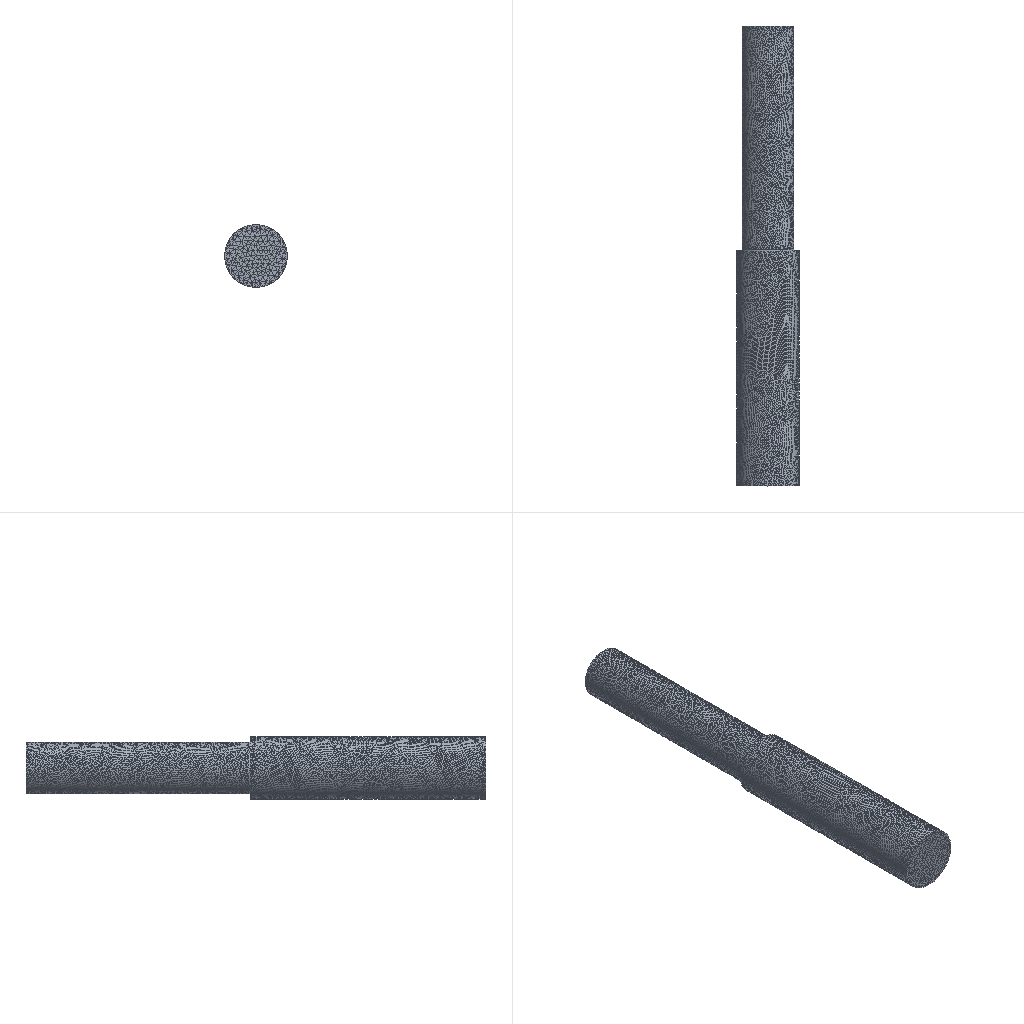Simulation study | ansys workbench
Set-up summary:
category,name,step,type,value,unit,region
solver,ansys_mapdl
solver,version,,,22.1
units,MPA,,stated
analysis,deck,,static,static
load_step,requested,,,1
analysis,nlgeom,,,False
mesh,nodes,,,113755
mesh,elements,,,65673
element_type,ANSYS 187 (type 1),,solid,65458
element_type,ANSYS 177 (type 2),,contact,76
element_type,ANSYS 170 (type 3),,target,0
element_type,ANSYS 177 (type 4),,contact,76
element_type,ANSYS 170 (type 5),,target,0
element_type,ANSYS 177 (type 6),,contact,63
element_type,ANSYS 170 (type 7),,target,0
load,load commands in deck,,count,9
bc,support commands in deck,,count,1
named_set,_FIXEDSU,,component
material,1,,in results
check,setup vs results,,match,results also hold 0 node(s) and 3 element(s) the deck makes with ['EN']; those were not compared; 3 node(s) the solver created internally for pilot nodes (ansys-fenxi-3/ansys有限元题目分析22/2_files/dp0/SYS-1/MECH/solve.out) are in the results only
Ansys APDL input file, long lists of numbers shortened:
/batch
/config,noeldb,1     ! force off writing results to database
*get,_wallstrt,active,,time,wall
! ANSYS input file written by Workbench version 2022 R1
! File used for geometry attach: F:\ansys（分析文件汇总)\ansys有限元题目分析\2_files\dp0\SYS-1\DM\SYS-1.scdoc
/title,2--____ (B5)
! ****** Begin Custom Load Command Snippet ******
/COM, ACT Extensions:
/COM,     LSDYNA, 2021.1
/COM,
! ****** End   Custom Load Command Snippet ******
*DIM,_wb_ProjectScratch_dir,string,248
_wb_ProjectScratch_dir(1) = 'F:\ansys（分析文件汇总)\ansys有限元题目分析\_ProjectScratch\Scr1AA7\'
*DIM,_wb_SolverFiles_dir,string,248
_wb_SolverFiles_dir(1) = 'F:\ansys（分析文件汇总)\ansys有限元题目分析\2_files\dp0\SYS-1\MECH\'
*DIM,_wb_userfiles_dir,string,248
_wb_userfiles_dir(1) = 'F:\ansys（分析文件汇总)\ansys有限元题目分析\2_files\user_files\'
/com,--- Data in consistent NMM units. See Solving Units in the help system for more information.
/units,MPA
/nopr
/wb,file,start              !  signify a WB generated input file
/prep7
! Turn off shape checking because checks already performed inside WB mesher.
! See help system for more information.
SHPP,OFF,,NOWARN
/nolist
etcon,set             ! allow ANSYS to choose best KEYOP's for 180x elements, resets any applicable keyopt to MAPDL defaults
/com,*********** Nodes for the whole assembly ***********
nblock,3,,125127
(1i9,3e20.9e3)
        1    -5.000000000E+01     4.541000000E+02    -2.832769449E-14
! (113751 more lines like these left out)
-1
/com,*********** Nodes for all Remote Points ***********
nblock,3
(1i9,3e20.9e3)
   113753     1.673250921E-03     0.000000000E+00     1.798580280E-16
   113754    -8.638767374E-16     4.405699968E+02     2.339666164E-16
   113755     1.382202767E-15     9.615300298E+02     2.159691824E-16
-1
/wb,elem,start            !  set before creation of elements
/com,*********** Elements for Body 1 "SYS-1\__" ***********
et,1,187
eblock,19,solid,,65458
(19i9)
        1        1        1        1        0        0        0        0       10        0        1     1404    17845    15600    17011    25846   106505    25844    25845
! (130915 more lines like these left out)
-1
/wb,elem,end               !  done creating elements
/com,*********** Send User Defined Coordinate System(s) ***********
csys,0
toffst,273.15,  ! Temperature offset from absolute zero
/com,*********** Set Reference Temperature ***********
tref,22.
/wb,mat,start              !  starting to send materials
/com,*********** Send Materials ***********
Temperature = 'TEMP' ! Temperature
MP,DENS,1,7.85e-09,	! tonne mm^-3
MP,ALPX,1,1.2e-05,	! C^-1
MP,C,1,434000000,	! mm^2 s^-2 C^-1
MP,KXX,1,60.5,	! tonne mm s^-3 C^-1
MP,RSVX,1,0.00017,	! ohm mm
MP,EX,1,200000,	! tonne s^-2 mm^-1
MP,NUXY,1,0.3,
MP,MURX,1,10000,
/wb,mat,end                !  done sending materials
!************************* Model Summary ********************
!SYS-1\__,	结构钢,	matid,	1
!************************* End Model Summary ********************
! get the diagonal of the bounding box. Needed later for other things
*get,_xmin,node,,mnloc,x
*get,_ymin,node,,mnloc,y
*get,_zmin,node,,mnloc,z
*get,_xmax,node,,mxloc,x
*get,_ymax,node,,mxloc,y
*get,_zmax,node,,mxloc,z
_ASMDIAG=(_xmax-_xmin)*(_xmax-_xmin)+(_ymax-_ymin)*(_ymax-_ymin)+(_zmax-_zmin)*(_zmax-_zmin)
_ASMDIAG=SQRT(_ASMDIAG)
/wb,contact,start          !  starting to send contact
/wb,contact,end            !  done creating contacts
/golist
/wb,load,start             !  starting to send loads
/com,*********** Fixed Supports ***********
CMBLOCK,_FIXEDSU,NODE,     1219
(8i10)
        64        65        66        67        68        69        70        71
! (152 more lines like these left out)
cmsel,s,_FIXEDSU
d,all,all
nsel,all
/com,*********** Create Remote Point "内部远程点" ***********
! -------- Remote Point Used by "力矩" --------
*set,tid,3
*set,cid,2
et,cid,177
et,tid,170
keyo,tid,2,1               ! Don't fix the pilot node
keyo,tid,4,111111
keyo,cid,12,5              ! Bonded Contact
keyo,cid,4,1               ! Deformable RBE3 style load
keyo,cid,2,2               ! MPC style contact
eblock,10,,,76
(15i9)
    90672        2        2        2        0      204      205    19196
! (75 more lines like these left out)
-1
*set,_npilot,113753
_npilot33=_npilot
type,tid
mat ,cid
real,cid
tshape,pilo
en,90748,_npilot
tshape
/com,*********** Create Remote Point "内部远程点 2" ***********
! -------- Remote Point Used by "力矩 2" --------
*set,tid,5
*set,cid,4
et,cid,177
et,tid,170
keyo,tid,2,1               ! Don't fix the pilot node
keyo,tid,4,111111
keyo,cid,12,5              ! Bonded Contact
keyo,cid,4,1               ! Deformable RBE3 style load
keyo,cid,2,2               ! MPC style contact
eblock,10,,,76
(15i9)
    90749        4        4        4        0      127      202    18846
! (75 more lines like these left out)
-1
*set,_npilot,113754
_npilot36=_npilot
type,tid
mat ,cid
real,cid
tshape,pilo
en,90825,_npilot
tshape
/com,*********** Create Remote Point "内部远程点 3" ***********
! -------- Remote Point Used by "力矩 3" --------
*set,tid,7
*set,cid,6
et,cid,177
et,tid,170
keyo,tid,2,1               ! Don't fix the pilot node
keyo,tid,4,111111
keyo,cid,12,5              ! Bonded Contact
keyo,cid,4,1               ! Deformable RBE3 style load
keyo,cid,2,2               ! MPC style contact
eblock,10,,,63
(15i9)
    90826        6        6        6        0       64       65    18501
! (62 more lines like these left out)
-1
*set,_npilot,113755
_npilot39=_npilot
type,tid
mat ,cid
real,cid
tshape,pilo
en,90889,_npilot
tshape
/com,*********** Construct Moment Using Remote Attachment ***********
/com,*********** Construct Moment Using Remote Attachment ***********
/com,*********** Construct Moment Using Remote Attachment ***********
/gst,on,on
fini
*get,_numnode,node,0,count
*get,_numelem,elem,0,count
*get, _MAXELEMNUM, elem, 0, NUM, MAX
*get, _MAXNODENUM, node, 0, NUM, MAX
*get, _MAXELEMTYPE, etyp, 0, NUM, MAX
*get, _MAXREALCONST, real, 0, NUM, MAX
/go
/wb,load,end               !  done creating loads
/com,--- Number of total nodes = %_numnode%
/com,--- Number of contact elements = 215
/com,--- Number of spring elements = 0
/com,--- Number of bearing elements = 0
/com,--- Number of solid elements = 65458
/com,--- Number of condensed parts = 0
/com,--- Number of total elements = %_numelem%
*get,_wallbsol,active,,time,wall
/com,****************************************************************************
/com,*************************    SOLUTION       ********************************
/com,****************************************************************************
/solu
antype,0                   ! static analysis
_thickRatio=  1     ! Ratio of thick parts in the model
eqsl,pcg,1e-8,,,,,,1
cntr,print,1               ! print out contact info and also make no initial contact an error
dmpoption,emat,no             ! Don't combine emat file for DANSYS
dmpoption,esav,no             ! Don't combine esav file for DANSYS
nldiag,cont,iter           ! print out contact info each equilibrium iteration
rescontrol,,none                 ! Do not keep any restart files
/com,****************************************************
/com,******************* SOLVE FOR LS 1 OF 1 ****************
nsel,s,node,,113753
f,all,mx,0.
f,all,my,-22000000.
f,all,mz,0.
nsel,s,node,,113754
f,all,mx,0.
f,all,my,-36000000.
f,all,mz,0.
nsel,s,node,,113755
f,all,mx,0.
f,all,my,-14000000.
f,all,mz,0.
nsel,all
/nopr
/gopr
nsub,1,1,1
time,1.
outres,erase
outres,all,none
outres,nsol,all,
outres,rsol,all
outres,eangl,all
outres,etmp,all
outres,veng,all
outres,strs,all,
outres,epel,all,
outres,eppl,all,
outres,cont,all,
! *********** WB SOLVE COMMAND ***********
! check interactive state
*get,ANSINTER_,active,,int
*if,ANSINTER_,ne,0,then
/eof
*endif
solve
/com *************** Write FE CONNECTORS *********
CEWRITE,file,ce,,INTE
/com,****************************************************
/com,*************** FINISHED SOLVE FOR LS 1 *************
*get,_wallasol,active,,time,wall
/nopr
*get,_numnode,node,0,count
*get,_numelem,elem,0,count
*get, _MAXELEMNUM, elem, 0, NUM, MAX
*get, _MAXNODENUM, node, 0, NUM, MAX,,,INTERNAL
*get, _MAXELEMTYPE, etyp, 0, NUM, MAX
*get, _MAXREALCONST, real, 0, NUM, MAX
/gopr
*get,_PCGITER,active,,solu,cgiter
/post1
xmlo,ENCODING,ISO-8859-1
xmlo,parm
/xml,parm,xml
fini
/gopr
*get,_walldone,active,,time,wall
_preptime=(_wallbsol-_wallstrt)*3600
_solvtime=(_wallasol-_wallbsol)*3600
_posttime=(_walldone-_wallasol)*3600
_totaltim=(_walldone-_wallstrt)*3600
*get,_dlbratio,active,0,solu,dlbr
*get,_combtime,active,0,solu,comb
*get,_ssmode,active,0,solu,ssmm
*get,_ndofs,active,0,solu,ndof
*get,_sol_end_time,active,0,set,time
*if,_sol_end_time,eq,1.,then
/fclean				!clean distributed files
*endif
/com,--- Total number of nodes = %_numnode%
/com,--- Total number of elements = %_numelem%
/com,--- Element load balance ratio = %_dlbratio%
/com,--- Time to combine distributed files = %_combtime%
/com,--- Sparse memory mode = %_ssmode%
/com,--- Number of DOF = %_ndofs%
/wb,file,end               ! done with WB generated input
Results summary:
result,analysis,,,static
result,last_loadstep,,,1
result,primary field,,,displacement
result,reaction total,1,FX,5.8e-05,N
result,reaction total,1,FY,0.000464,N
result,reaction total,1,FZ,-0.000861,N
result,mass,,,0.0669,"NMM: mm, ton, N, s, mV, mA, degC"